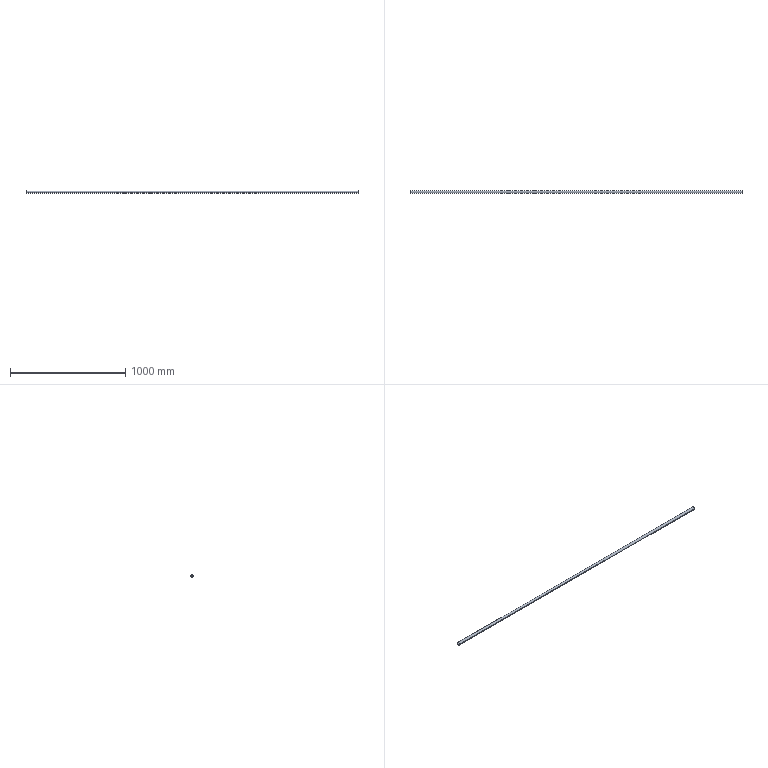Part | STEP file | 粉仓楼梯通道护栏1栏杆_Default<As Machined> | 1 solid | 6 faces | box 2880 x 25 x 25 mm | volume 318934 mm3 | cylinder 4 | plane 2 | commonest cylinder face diameters 22 x2 25 x2
STEP:
#1=CARTESIAN_POINT('',(0.,0.,0.));
#2=DIRECTION('',(0.,0.,1.));
#3=DIRECTION('',(1.,0.,0.));
#4=AXIS2_PLACEMENT_3D('',#1,#2,#3);
#5=CARTESIAN_POINT('',(1440.,12.5,0.));
#6=VERTEX_POINT('',#5);
#7=CARTESIAN_POINT('',(1440.,-12.5,0.));
#8=VERTEX_POINT('',#7);
#9=CARTESIAN_POINT('',(1440.,0.,0.));
#10=DIRECTION('',(1.,0.,0.));
#11=DIRECTION('',(0.,1.,0.));
#12=AXIS2_PLACEMENT_3D('',#9,#10,#11);
#13=CIRCLE('',#12,12.5);
#14=CARTESIAN_POINT('',(1440.,0.,0.));
#15=DIRECTION('',(-1.,0.,0.));
#16=DIRECTION('',(0.,-1.,0.));
#17=AXIS2_PLACEMENT_3D('',#14,#15,#16);
#18=CYLINDRICAL_SURFACE('',#17,12.5);
#19=CARTESIAN_POINT('',(3.142,0.));
#20=DIRECTION('',(-1.,0.));
#21=VECTOR('',#20,1.);
#22=LINE('',#19,#21);
#23=(GEOMETRIC_REPRESENTATION_CONTEXT(2)PARAMETRIC_REPRESENTATION_CONTEXT()REPRESENTATION_CONTEXT('',''));
#24=DEFINITIONAL_REPRESENTATION('',(#22),#23);
#25=PCURVE('',#18,#24);
#26=CARTESIAN_POINT('',(1440.,0.,0.));
#27=DIRECTION('',(1.,0.,0.));
#28=DIRECTION('',(0.,1.,0.));
#29=AXIS2_PLACEMENT_3D('',#26,#27,#28);
#30=PLANE('',#29);
#31=CARTESIAN_POINT('',(0.,0.));
#32=DIRECTION('',(1.,0.));
#33=AXIS2_PLACEMENT_2D('',#31,#32);
#34=CIRCLE('',#33,12.5);
#35=(GEOMETRIC_REPRESENTATION_CONTEXT(2)PARAMETRIC_REPRESENTATION_CONTEXT()REPRESENTATION_CONTEXT('',''));
#36=DEFINITIONAL_REPRESENTATION('',(#34),#35);
#37=PCURVE('',#30,#36);
#38=SURFACE_CURVE('',#13,(#25,#37),.PCURVE_S1.);
#39=EDGE_CURVE('',#6,#8,#38,.T.);
#40=ORIENTED_EDGE('',*,*,#39,.F.);
#41=CARTESIAN_POINT('',(-1440.,12.5,0.));
#42=VERTEX_POINT('',#41);
#43=CARTESIAN_POINT('',(1440.,12.5,0.));
#44=DIRECTION('',(-1.,0.,0.));
#45=VECTOR('',#44,1.);
#46=LINE('',#43,#45);
#47=CARTESIAN_POINT('',(3.142,0.));
#48=DIRECTION('',(0.,1.));
#49=VECTOR('',#48,1.);
#50=LINE('',#47,#49);
#51=(GEOMETRIC_REPRESENTATION_CONTEXT(2)PARAMETRIC_REPRESENTATION_CONTEXT()REPRESENTATION_CONTEXT('',''));
#52=DEFINITIONAL_REPRESENTATION('',(#50),#51);
#53=PCURVE('',#18,#52);
#54=CARTESIAN_POINT('',(1440.,0.,0.));
#55=DIRECTION('',(-1.,0.,0.));
#56=DIRECTION('',(0.,-1.,0.));
#57=AXIS2_PLACEMENT_3D('',#54,#55,#56);
#58=CYLINDRICAL_SURFACE('',#57,12.5);
#59=CARTESIAN_POINT('',(3.142,0.));
#60=DIRECTION('',(0.,1.));
#61=VECTOR('',#60,1.);
#62=LINE('',#59,#61);
#63=(GEOMETRIC_REPRESENTATION_CONTEXT(2)PARAMETRIC_REPRESENTATION_CONTEXT()REPRESENTATION_CONTEXT('',''));
#64=DEFINITIONAL_REPRESENTATION('',(#62),#63);
#65=PCURVE('',#58,#64);
#66=SURFACE_CURVE('',#46,(#53,#65),.PCURVE_S1.);
#67=EDGE_CURVE('',#6,#42,#66,.T.);
#68=ORIENTED_EDGE('',*,*,#67,.T.);
#69=CARTESIAN_POINT('',(-1440.,-12.5,0.));
#70=VERTEX_POINT('',#69);
#71=CARTESIAN_POINT('',(-1440.,0.,0.));
#72=DIRECTION('',(1.,0.,0.));
#73=DIRECTION('',(0.,1.,0.));
#74=AXIS2_PLACEMENT_3D('',#71,#72,#73);
#75=CIRCLE('',#74,12.5);
#76=CARTESIAN_POINT('',(3.142,2880.));
#77=DIRECTION('',(-1.,0.));
#78=VECTOR('',#77,1.);
#79=LINE('',#76,#78);
#80=(GEOMETRIC_REPRESENTATION_CONTEXT(2)PARAMETRIC_REPRESENTATION_CONTEXT()REPRESENTATION_CONTEXT('',''));
#81=DEFINITIONAL_REPRESENTATION('',(#79),#80);
#82=PCURVE('',#18,#81);
#83=CARTESIAN_POINT('',(-1440.,0.,0.));
#84=DIRECTION('',(1.,0.,0.));
#85=DIRECTION('',(0.,1.,0.));
#86=AXIS2_PLACEMENT_3D('',#83,#84,#85);
#87=PLANE('',#86);
#88=CARTESIAN_POINT('',(0.,0.));
#89=DIRECTION('',(1.,0.));
#90=AXIS2_PLACEMENT_2D('',#88,#89);
#91=CIRCLE('',#90,12.5);
#92=(GEOMETRIC_REPRESENTATION_CONTEXT(2)PARAMETRIC_REPRESENTATION_CONTEXT()REPRESENTATION_CONTEXT('',''));
#93=DEFINITIONAL_REPRESENTATION('',(#91),#92);
#94=PCURVE('',#87,#93);
#95=SURFACE_CURVE('',#75,(#82,#94),.PCURVE_S1.);
#96=EDGE_CURVE('',#42,#70,#95,.T.);
#97=ORIENTED_EDGE('',*,*,#96,.T.);
#98=CARTESIAN_POINT('',(1440.,-12.5,0.));
#99=DIRECTION('',(-1.,0.,0.));
#100=VECTOR('',#99,1.);
#101=LINE('',#98,#100);
#102=CARTESIAN_POINT('',(0.,0.));
#103=DIRECTION('',(0.,1.));
#104=VECTOR('',#103,1.);
#105=LINE('',#102,#104);
#106=(GEOMETRIC_REPRESENTATION_CONTEXT(2)PARAMETRIC_REPRESENTATION_CONTEXT()REPRESENTATION_CONTEXT('',''));
#107=DEFINITIONAL_REPRESENTATION('',(#105),#106);
#108=PCURVE('',#18,#107);
#109=CARTESIAN_POINT('',(6.283,0.));
#110=DIRECTION('',(0.,1.));
#111=VECTOR('',#110,1.);
#112=LINE('',#109,#111);
#113=(GEOMETRIC_REPRESENTATION_CONTEXT(2)PARAMETRIC_REPRESENTATION_CONTEXT()REPRESENTATION_CONTEXT('',''));
#114=DEFINITIONAL_REPRESENTATION('',(#112),#113);
#115=PCURVE('',#58,#114);
#116=SURFACE_CURVE('',#101,(#108,#115),.PCURVE_S1.);
#117=EDGE_CURVE('',#8,#70,#116,.T.);
#118=ORIENTED_EDGE('',*,*,#117,.F.);
#119=EDGE_LOOP('',(#40,#68,#97,#118));
#120=FACE_BOUND('',#119,.T.);
#121=ADVANCED_FACE('',(#120),#18,.T.);
#122=CARTESIAN_POINT('',(1440.,-11.,0.));
#123=VERTEX_POINT('',#122);
#124=CARTESIAN_POINT('',(-1440.,-11.,0.));
#125=VERTEX_POINT('',#124);
#126=CARTESIAN_POINT('',(1440.,-11.,0.));
#127=DIRECTION('',(-1.,0.,0.));
#128=VECTOR('',#127,1.);
#129=LINE('',#126,#128);
#130=CARTESIAN_POINT('',(1440.,0.,0.));
#131=DIRECTION('',(-1.,0.,0.));
#132=DIRECTION('',(0.,-1.,0.));
#133=AXIS2_PLACEMENT_3D('',#130,#131,#132);
#134=CYLINDRICAL_SURFACE('',#133,11.);
#135=CARTESIAN_POINT('',(6.283,0.));
#136=DIRECTION('',(0.,1.));
#137=VECTOR('',#136,1.);
#138=LINE('',#135,#137);
#139=(GEOMETRIC_REPRESENTATION_CONTEXT(2)PARAMETRIC_REPRESENTATION_CONTEXT()REPRESENTATION_CONTEXT('',''));
#140=DEFINITIONAL_REPRESENTATION('',(#138),#139);
#141=PCURVE('',#134,#140);
#142=CARTESIAN_POINT('',(1440.,0.,0.));
#143=DIRECTION('',(-1.,0.,0.));
#144=DIRECTION('',(0.,-1.,0.));
#145=AXIS2_PLACEMENT_3D('',#142,#143,#144);
#146=CYLINDRICAL_SURFACE('',#145,11.);
#147=CARTESIAN_POINT('',(0.,0.));
#148=DIRECTION('',(0.,1.));
#149=VECTOR('',#148,1.);
#150=LINE('',#147,#149);
#151=(GEOMETRIC_REPRESENTATION_CONTEXT(2)PARAMETRIC_REPRESENTATION_CONTEXT()REPRESENTATION_CONTEXT('',''));
#152=DEFINITIONAL_REPRESENTATION('',(#150),#151);
#153=PCURVE('',#146,#152);
#154=SURFACE_CURVE('',#129,(#141,#153),.PCURVE_S1.);
#155=EDGE_CURVE('',#123,#125,#154,.T.);
#156=ORIENTED_EDGE('',*,*,#155,.T.);
#157=CARTESIAN_POINT('',(-1440.,11.,0.));
#158=VERTEX_POINT('',#157);
#159=CARTESIAN_POINT('',(-1440.,0.,0.));
#160=DIRECTION('',(1.,0.,0.));
#161=DIRECTION('',(0.,1.,0.));
#162=AXIS2_PLACEMENT_3D('',#159,#160,#161);
#163=CIRCLE('',#162,11.);
#164=CARTESIAN_POINT('',(9.425,2880.));
#165=DIRECTION('',(-1.,0.));
#166=VECTOR('',#165,1.);
#167=LINE('',#164,#166);
#168=(GEOMETRIC_REPRESENTATION_CONTEXT(2)PARAMETRIC_REPRESENTATION_CONTEXT()REPRESENTATION_CONTEXT('',''));
#169=DEFINITIONAL_REPRESENTATION('',(#167),#168);
#170=PCURVE('',#134,#169);
#171=CARTESIAN_POINT('',(0.,0.));
#172=DIRECTION('',(1.,0.));
#173=AXIS2_PLACEMENT_2D('',#171,#172);
#174=CIRCLE('',#173,11.);
#175=(GEOMETRIC_REPRESENTATION_CONTEXT(2)PARAMETRIC_REPRESENTATION_CONTEXT()REPRESENTATION_CONTEXT('',''));
#176=DEFINITIONAL_REPRESENTATION('',(#174),#175);
#177=PCURVE('',#87,#176);
#178=SURFACE_CURVE('',#163,(#170,#177),.PCURVE_S1.);
#179=EDGE_CURVE('',#125,#158,#178,.T.);
#180=ORIENTED_EDGE('',*,*,#179,.T.);
#181=CARTESIAN_POINT('',(1440.,11.,0.));
#182=VERTEX_POINT('',#181);
#183=CARTESIAN_POINT('',(1440.,11.,0.));
#184=DIRECTION('',(-1.,0.,0.));
#185=VECTOR('',#184,1.);
#186=LINE('',#183,#185);
#187=CARTESIAN_POINT('',(3.142,0.));
#188=DIRECTION('',(0.,1.));
#189=VECTOR('',#188,1.);
#190=LINE('',#187,#189);
#191=(GEOMETRIC_REPRESENTATION_CONTEXT(2)PARAMETRIC_REPRESENTATION_CONTEXT()REPRESENTATION_CONTEXT('',''));
#192=DEFINITIONAL_REPRESENTATION('',(#190),#191);
#193=PCURVE('',#134,#192);
#194=CARTESIAN_POINT('',(3.142,0.));
#195=DIRECTION('',(0.,1.));
#196=VECTOR('',#195,1.);
#197=LINE('',#194,#196);
#198=(GEOMETRIC_REPRESENTATION_CONTEXT(2)PARAMETRIC_REPRESENTATION_CONTEXT()REPRESENTATION_CONTEXT('',''));
#199=DEFINITIONAL_REPRESENTATION('',(#197),#198);
#200=PCURVE('',#146,#199);
#201=SURFACE_CURVE('',#186,(#193,#200),.PCURVE_S1.);
#202=EDGE_CURVE('',#182,#158,#201,.T.);
#203=ORIENTED_EDGE('',*,*,#202,.F.);
#204=CARTESIAN_POINT('',(1440.,0.,0.));
#205=DIRECTION('',(1.,0.,0.));
#206=DIRECTION('',(0.,1.,0.));
#207=AXIS2_PLACEMENT_3D('',#204,#205,#206);
#208=CIRCLE('',#207,11.);
#209=CARTESIAN_POINT('',(9.425,0.));
#210=DIRECTION('',(-1.,0.));
#211=VECTOR('',#210,1.);
#212=LINE('',#209,#211);
#213=(GEOMETRIC_REPRESENTATION_CONTEXT(2)PARAMETRIC_REPRESENTATION_CONTEXT()REPRESENTATION_CONTEXT('',''));
#214=DEFINITIONAL_REPRESENTATION('',(#212),#213);
#215=PCURVE('',#134,#214);
#216=CARTESIAN_POINT('',(0.,0.));
#217=DIRECTION('',(1.,0.));
#218=AXIS2_PLACEMENT_2D('',#216,#217);
#219=CIRCLE('',#218,11.);
#220=(GEOMETRIC_REPRESENTATION_CONTEXT(2)PARAMETRIC_REPRESENTATION_CONTEXT()REPRESENTATION_CONTEXT('',''));
#221=DEFINITIONAL_REPRESENTATION('',(#219),#220);
#222=PCURVE('',#30,#221);
#223=SURFACE_CURVE('',#208,(#215,#222),.PCURVE_S1.);
#224=EDGE_CURVE('',#123,#182,#223,.T.);
#225=ORIENTED_EDGE('',*,*,#224,.F.);
#226=EDGE_LOOP('',(#156,#180,#203,#225));
#227=FACE_BOUND('',#226,.F.);
#228=ADVANCED_FACE('',(#227),#134,.F.);
#229=CARTESIAN_POINT('',(-1440.,0.,0.));
#230=DIRECTION('',(1.,0.,0.));
#231=DIRECTION('',(0.,1.,0.));
#232=AXIS2_PLACEMENT_3D('',#229,#230,#231);
#233=CIRCLE('',#232,11.);
#234=CARTESIAN_POINT('',(3.142,2880.));
#235=DIRECTION('',(-1.,0.));
#236=VECTOR('',#235,1.);
#237=LINE('',#234,#236);
#238=(GEOMETRIC_REPRESENTATION_CONTEXT(2)PARAMETRIC_REPRESENTATION_CONTEXT()REPRESENTATION_CONTEXT('',''));
#239=DEFINITIONAL_REPRESENTATION('',(#237),#238);
#240=PCURVE('',#146,#239);
#241=CARTESIAN_POINT('',(0.,0.));
#242=DIRECTION('',(1.,0.));
#243=AXIS2_PLACEMENT_2D('',#241,#242);
#244=CIRCLE('',#243,11.);
#245=(GEOMETRIC_REPRESENTATION_CONTEXT(2)PARAMETRIC_REPRESENTATION_CONTEXT()REPRESENTATION_CONTEXT('',''));
#246=DEFINITIONAL_REPRESENTATION('',(#244),#245);
#247=PCURVE('',#87,#246);
#248=SURFACE_CURVE('',#233,(#240,#247),.PCURVE_S1.);
#249=EDGE_CURVE('',#158,#125,#248,.T.);
#250=ORIENTED_EDGE('',*,*,#249,.T.);
#251=ORIENTED_EDGE('',*,*,#155,.F.);
#252=CARTESIAN_POINT('',(1440.,0.,0.));
#253=DIRECTION('',(1.,0.,0.));
#254=DIRECTION('',(0.,1.,0.));
#255=AXIS2_PLACEMENT_3D('',#252,#253,#254);
#256=CIRCLE('',#255,11.);
#257=CARTESIAN_POINT('',(3.142,0.));
#258=DIRECTION('',(-1.,0.));
#259=VECTOR('',#258,1.);
#260=LINE('',#257,#259);
#261=(GEOMETRIC_REPRESENTATION_CONTEXT(2)PARAMETRIC_REPRESENTATION_CONTEXT()REPRESENTATION_CONTEXT('',''));
#262=DEFINITIONAL_REPRESENTATION('',(#260),#261);
#263=PCURVE('',#146,#262);
#264=CARTESIAN_POINT('',(0.,0.));
#265=DIRECTION('',(1.,0.));
#266=AXIS2_PLACEMENT_2D('',#264,#265);
#267=CIRCLE('',#266,11.);
#268=(GEOMETRIC_REPRESENTATION_CONTEXT(2)PARAMETRIC_REPRESENTATION_CONTEXT()REPRESENTATION_CONTEXT('',''));
#269=DEFINITIONAL_REPRESENTATION('',(#267),#268);
#270=PCURVE('',#30,#269);
#271=SURFACE_CURVE('',#256,(#263,#270),.PCURVE_S1.);
#272=EDGE_CURVE('',#182,#123,#271,.T.);
#273=ORIENTED_EDGE('',*,*,#272,.F.);
#274=ORIENTED_EDGE('',*,*,#202,.T.);
#275=EDGE_LOOP('',(#250,#251,#273,#274));
#276=FACE_BOUND('',#275,.F.);
#277=ADVANCED_FACE('',(#276),#146,.F.);
#278=ORIENTED_EDGE('',*,*,#67,.F.);
#279=CARTESIAN_POINT('',(1440.,0.,0.));
#280=DIRECTION('',(1.,0.,0.));
#281=DIRECTION('',(0.,1.,0.));
#282=AXIS2_PLACEMENT_3D('',#279,#280,#281);
#283=CIRCLE('',#282,12.5);
#284=CARTESIAN_POINT('',(9.425,0.));
#285=DIRECTION('',(-1.,0.));
#286=VECTOR('',#285,1.);
#287=LINE('',#284,#286);
#288=(GEOMETRIC_REPRESENTATION_CONTEXT(2)PARAMETRIC_REPRESENTATION_CONTEXT()REPRESENTATION_CONTEXT('',''));
#289=DEFINITIONAL_REPRESENTATION('',(#287),#288);
#290=PCURVE('',#58,#289);
#291=CARTESIAN_POINT('',(0.,0.));
#292=DIRECTION('',(1.,0.));
#293=AXIS2_PLACEMENT_2D('',#291,#292);
#294=CIRCLE('',#293,12.5);
#295=(GEOMETRIC_REPRESENTATION_CONTEXT(2)PARAMETRIC_REPRESENTATION_CONTEXT()REPRESENTATION_CONTEXT('',''));
#296=DEFINITIONAL_REPRESENTATION('',(#294),#295);
#297=PCURVE('',#30,#296);
#298=SURFACE_CURVE('',#283,(#290,#297),.PCURVE_S1.);
#299=EDGE_CURVE('',#8,#6,#298,.T.);
#300=ORIENTED_EDGE('',*,*,#299,.F.);
#301=ORIENTED_EDGE('',*,*,#117,.T.);
#302=CARTESIAN_POINT('',(-1440.,0.,0.));
#303=DIRECTION('',(1.,0.,0.));
#304=DIRECTION('',(0.,1.,0.));
#305=AXIS2_PLACEMENT_3D('',#302,#303,#304);
#306=CIRCLE('',#305,12.5);
#307=CARTESIAN_POINT('',(9.425,2880.));
#308=DIRECTION('',(-1.,0.));
#309=VECTOR('',#308,1.);
#310=LINE('',#307,#309);
#311=(GEOMETRIC_REPRESENTATION_CONTEXT(2)PARAMETRIC_REPRESENTATION_CONTEXT()REPRESENTATION_CONTEXT('',''));
#312=DEFINITIONAL_REPRESENTATION('',(#310),#311);
#313=PCURVE('',#58,#312);
#314=CARTESIAN_POINT('',(0.,0.));
#315=DIRECTION('',(1.,0.));
#316=AXIS2_PLACEMENT_2D('',#314,#315);
#317=CIRCLE('',#316,12.5);
#318=(GEOMETRIC_REPRESENTATION_CONTEXT(2)PARAMETRIC_REPRESENTATION_CONTEXT()REPRESENTATION_CONTEXT('',''));
#319=DEFINITIONAL_REPRESENTATION('',(#317),#318);
#320=PCURVE('',#87,#319);
#321=SURFACE_CURVE('',#306,(#313,#320),.PCURVE_S1.);
#322=EDGE_CURVE('',#70,#42,#321,.T.);
#323=ORIENTED_EDGE('',*,*,#322,.T.);
#324=EDGE_LOOP('',(#278,#300,#301,#323));
#325=FACE_BOUND('',#324,.T.);
#326=ADVANCED_FACE('',(#325),#58,.T.);
#327=ORIENTED_EDGE('',*,*,#224,.F.);
#328=ORIENTED_EDGE('',*,*,#272,.F.);
#329=EDGE_LOOP('',(#327,#328));
#330=FACE_BOUND('',#329,.T.);
#331=ORIENTED_EDGE('',*,*,#299,.T.);
#332=ORIENTED_EDGE('',*,*,#39,.T.);
#333=EDGE_LOOP('',(#331,#332));
#334=FACE_BOUND('',#333,.T.);
#335=ADVANCED_FACE('',(#330,#334),#30,.T.);
#336=ORIENTED_EDGE('',*,*,#179,.T.);
#337=ORIENTED_EDGE('',*,*,#249,.T.);
#338=EDGE_LOOP('',(#336,#337));
#339=FACE_BOUND('',#338,.T.);
#340=ORIENTED_EDGE('',*,*,#322,.F.);
#341=ORIENTED_EDGE('',*,*,#96,.F.);
#342=EDGE_LOOP('',(#340,#341));
#343=FACE_BOUND('',#342,.T.);
#344=ADVANCED_FACE('',(#339,#343),#87,.F.);
#345=CLOSED_SHELL('',(#121,#228,#277,#326,#335,#344));
#346=MANIFOLD_SOLID_BREP('',#345);
#347=(LENGTH_UNIT()NAMED_UNIT(*)SI_UNIT(.MILLI.,.METRE.));
#348=UNCERTAINTY_MEASURE_WITH_UNIT(LENGTH_MEASURE(0.0000001),#347,'','');
#349=(NAMED_UNIT(*)PLANE_ANGLE_UNIT()SI_UNIT($,.RADIAN.));
#350=(NAMED_UNIT(*)SI_UNIT($,.STERADIAN.)SOLID_ANGLE_UNIT());
#351=(GEOMETRIC_REPRESENTATION_CONTEXT(3)GLOBAL_UNCERTAINTY_ASSIGNED_CONTEXT((#348))GLOBAL_UNIT_ASSIGNED_CONTEXT((#347,#349,#350))REPRESENTATION_CONTEXT('',''));
#352=ADVANCED_BREP_SHAPE_REPRESENTATION('',(#4,#346),#351);